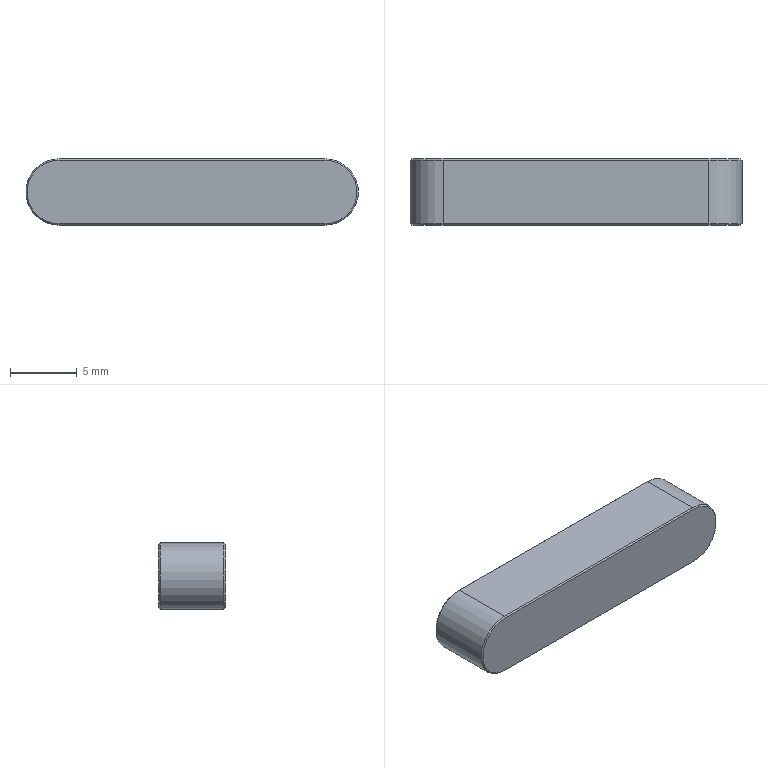Part | STEP file | Plain key type A 5x5x25 | 1 solid | 14 faces | box 25 x 5 x 5 mm | volume 597.62 mm3 | plane 8 | cone 4 | cylinder 2 | commonest cylinder face diameters 5 x2
STEP:
#1=CARTESIAN_POINT('',(0.,0.,0.));
#2=DIRECTION('',(0.,0.,1.));
#3=DIRECTION('',(1.,0.,0.));
#4=AXIS2_PLACEMENT_3D('',#1,#2,#3);
#5=CARTESIAN_POINT('',(-10.,2.4,-2.5));
#6=VERTEX_POINT('',#5);
#7=CARTESIAN_POINT('',(-10.,-2.4,-2.5));
#8=VERTEX_POINT('',#7);
#9=CARTESIAN_POINT('',(-10.,2.5,-2.5));
#10=DIRECTION('',(0.,-1.,0.));
#11=VECTOR('',#10,1.);
#12=LINE('',#9,#11);
#13=CARTESIAN_POINT('',(-10.,2.5,0.));
#14=DIRECTION('',(0.,-1.,0.));
#15=DIRECTION('',(0.,0.,-1.));
#16=AXIS2_PLACEMENT_3D('',#13,#14,#15);
#17=CYLINDRICAL_SURFACE('',#16,2.5);
#18=CARTESIAN_POINT('',(6.283,0.));
#19=DIRECTION('',(0.,1.));
#20=VECTOR('',#19,1.);
#21=LINE('',#18,#20);
#22=(GEOMETRIC_REPRESENTATION_CONTEXT(2)PARAMETRIC_REPRESENTATION_CONTEXT()REPRESENTATION_CONTEXT('',''));
#23=DEFINITIONAL_REPRESENTATION('',(#21),#22);
#24=PCURVE('',#17,#23);
#25=CARTESIAN_POINT('',(-10.,2.5,-2.5));
#26=DIRECTION('',(0.,0.,1.));
#27=DIRECTION('',(1.,0.,0.));
#28=AXIS2_PLACEMENT_3D('',#25,#26,#27);
#29=PLANE('',#28);
#30=CARTESIAN_POINT('',(0.,0.));
#31=DIRECTION('',(0.,-1.));
#32=VECTOR('',#31,1.);
#33=LINE('',#30,#32);
#34=(GEOMETRIC_REPRESENTATION_CONTEXT(2)PARAMETRIC_REPRESENTATION_CONTEXT()REPRESENTATION_CONTEXT('',''));
#35=DEFINITIONAL_REPRESENTATION('',(#33),#34);
#36=PCURVE('',#29,#35);
#37=SURFACE_CURVE('',#12,(#24,#36),.PCURVE_S1.);
#38=EDGE_CURVE('',#6,#8,#37,.T.);
#39=ORIENTED_EDGE('',*,*,#38,.T.);
#40=CARTESIAN_POINT('',(-10.,-2.4,2.5));
#41=VERTEX_POINT('',#40);
#42=CARTESIAN_POINT('',(-10.,-2.4,0.));
#43=DIRECTION('',(0.,1.,0.));
#44=DIRECTION('',(0.,0.,1.));
#45=AXIS2_PLACEMENT_3D('',#42,#43,#44);
#46=CIRCLE('',#45,2.5);
#47=CARTESIAN_POINT('',(9.425,4.9));
#48=DIRECTION('',(-1.,0.));
#49=VECTOR('',#48,1.);
#50=LINE('',#47,#49);
#51=(GEOMETRIC_REPRESENTATION_CONTEXT(2)PARAMETRIC_REPRESENTATION_CONTEXT()REPRESENTATION_CONTEXT('',''));
#52=DEFINITIONAL_REPRESENTATION('',(#50),#51);
#53=PCURVE('',#17,#52);
#54=CARTESIAN_POINT('',(-10.,-2.4,0.));
#55=DIRECTION('',(0.,1.,0.));
#56=DIRECTION('',(0.,0.,1.));
#57=AXIS2_PLACEMENT_3D('',#54,#55,#56);
#58=CONICAL_SURFACE('',#57,2.5,0.7854);
#59=CARTESIAN_POINT('',(0.,0.));
#60=DIRECTION('',(1.,0.));
#61=VECTOR('',#60,1.);
#62=LINE('',#59,#61);
#63=(GEOMETRIC_REPRESENTATION_CONTEXT(2)PARAMETRIC_REPRESENTATION_CONTEXT()REPRESENTATION_CONTEXT('',''));
#64=DEFINITIONAL_REPRESENTATION('',(#62),#63);
#65=PCURVE('',#58,#64);
#66=SURFACE_CURVE('',#46,(#53,#65),.PCURVE_S1.);
#67=EDGE_CURVE('',#8,#41,#66,.T.);
#68=ORIENTED_EDGE('',*,*,#67,.T.);
#69=CARTESIAN_POINT('',(-10.,2.4,2.5));
#70=VERTEX_POINT('',#69);
#71=CARTESIAN_POINT('',(-10.,2.5,2.5));
#72=DIRECTION('',(0.,-1.,0.));
#73=VECTOR('',#72,1.);
#74=LINE('',#71,#73);
#75=CARTESIAN_POINT('',(3.142,0.));
#76=DIRECTION('',(0.,1.));
#77=VECTOR('',#76,1.);
#78=LINE('',#75,#77);
#79=(GEOMETRIC_REPRESENTATION_CONTEXT(2)PARAMETRIC_REPRESENTATION_CONTEXT()REPRESENTATION_CONTEXT('',''));
#80=DEFINITIONAL_REPRESENTATION('',(#78),#79);
#81=PCURVE('',#17,#80);
#82=CARTESIAN_POINT('',(-10.,2.5,2.5));
#83=DIRECTION('',(0.,0.,-1.));
#84=DIRECTION('',(-1.,0.,0.));
#85=AXIS2_PLACEMENT_3D('',#82,#83,#84);
#86=PLANE('',#85);
#87=CARTESIAN_POINT('',(0.,0.));
#88=DIRECTION('',(0.,-1.));
#89=VECTOR('',#88,1.);
#90=LINE('',#87,#89);
#91=(GEOMETRIC_REPRESENTATION_CONTEXT(2)PARAMETRIC_REPRESENTATION_CONTEXT()REPRESENTATION_CONTEXT('',''));
#92=DEFINITIONAL_REPRESENTATION('',(#90),#91);
#93=PCURVE('',#86,#92);
#94=SURFACE_CURVE('',#74,(#81,#93),.PCURVE_S1.);
#95=EDGE_CURVE('',#70,#41,#94,.T.);
#96=ORIENTED_EDGE('',*,*,#95,.F.);
#97=CARTESIAN_POINT('',(-10.,2.4,0.));
#98=DIRECTION('',(0.,-1.,0.));
#99=DIRECTION('',(0.,0.,1.));
#100=AXIS2_PLACEMENT_3D('',#97,#98,#99);
#101=CIRCLE('',#100,2.5);
#102=CARTESIAN_POINT('',(3.142,0.1));
#103=DIRECTION('',(1.,0.));
#104=VECTOR('',#103,1.);
#105=LINE('',#102,#104);
#106=(GEOMETRIC_REPRESENTATION_CONTEXT(2)PARAMETRIC_REPRESENTATION_CONTEXT()REPRESENTATION_CONTEXT('',''));
#107=DEFINITIONAL_REPRESENTATION('',(#105),#106);
#108=PCURVE('',#17,#107);
#109=CARTESIAN_POINT('',(-10.,2.5,0.));
#110=DIRECTION('',(0.,-1.,0.));
#111=DIRECTION('',(0.,0.,-1.));
#112=AXIS2_PLACEMENT_3D('',#109,#110,#111);
#113=CONICAL_SURFACE('',#112,2.4,0.7854);
#114=CARTESIAN_POINT('',(3.142,0.1));
#115=DIRECTION('',(1.,0.));
#116=VECTOR('',#115,1.);
#117=LINE('',#114,#116);
#118=(GEOMETRIC_REPRESENTATION_CONTEXT(2)PARAMETRIC_REPRESENTATION_CONTEXT()REPRESENTATION_CONTEXT('',''));
#119=DEFINITIONAL_REPRESENTATION('',(#117),#118);
#120=PCURVE('',#113,#119);
#121=SURFACE_CURVE('',#101,(#108,#120),.PCURVE_S1.);
#122=EDGE_CURVE('',#70,#6,#121,.T.);
#123=ORIENTED_EDGE('',*,*,#122,.T.);
#124=EDGE_LOOP('',(#39,#68,#96,#123));
#125=FACE_BOUND('',#124,.T.);
#126=ADVANCED_FACE('',(#125),#17,.T.);
#127=ORIENTED_EDGE('',*,*,#95,.T.);
#128=CARTESIAN_POINT('',(10.,-2.4,2.5));
#129=VERTEX_POINT('',#128);
#130=CARTESIAN_POINT('',(-10.,-2.4,2.5));
#131=DIRECTION('',(1.,0.,0.));
#132=VECTOR('',#131,1.);
#133=LINE('',#130,#132);
#134=CARTESIAN_POINT('',(0.,-4.9));
#135=DIRECTION('',(-1.,0.));
#136=VECTOR('',#135,1.);
#137=LINE('',#134,#136);
#138=(GEOMETRIC_REPRESENTATION_CONTEXT(2)PARAMETRIC_REPRESENTATION_CONTEXT()REPRESENTATION_CONTEXT('',''));
#139=DEFINITIONAL_REPRESENTATION('',(#137),#138);
#140=PCURVE('',#86,#139);
#141=CARTESIAN_POINT('',(-10.,-2.4,2.5));
#142=DIRECTION('',(0.,0.7071,-0.7071));
#143=DIRECTION('',(1.,0.,0.));
#144=AXIS2_PLACEMENT_3D('',#141,#142,#143);
#145=PLANE('',#144);
#146=CARTESIAN_POINT('',(0.,0.));
#147=DIRECTION('',(1.,0.));
#148=VECTOR('',#147,1.);
#149=LINE('',#146,#148);
#150=(GEOMETRIC_REPRESENTATION_CONTEXT(2)PARAMETRIC_REPRESENTATION_CONTEXT()REPRESENTATION_CONTEXT('',''));
#151=DEFINITIONAL_REPRESENTATION('',(#149),#150);
#152=PCURVE('',#145,#151);
#153=SURFACE_CURVE('',#133,(#140,#152),.PCURVE_S1.);
#154=EDGE_CURVE('',#41,#129,#153,.T.);
#155=ORIENTED_EDGE('',*,*,#154,.T.);
#156=CARTESIAN_POINT('',(10.,2.4,2.5));
#157=VERTEX_POINT('',#156);
#158=CARTESIAN_POINT('',(10.,2.5,2.5));
#159=DIRECTION('',(0.,-1.,0.));
#160=VECTOR('',#159,1.);
#161=LINE('',#158,#160);
#162=CARTESIAN_POINT('',(-20.,0.));
#163=DIRECTION('',(0.,-1.));
#164=VECTOR('',#163,1.);
#165=LINE('',#162,#164);
#166=(GEOMETRIC_REPRESENTATION_CONTEXT(2)PARAMETRIC_REPRESENTATION_CONTEXT()REPRESENTATION_CONTEXT('',''));
#167=DEFINITIONAL_REPRESENTATION('',(#165),#166);
#168=PCURVE('',#86,#167);
#169=CARTESIAN_POINT('',(10.,2.5,0.));
#170=DIRECTION('',(0.,-1.,0.));
#171=DIRECTION('',(0.,0.,-1.));
#172=AXIS2_PLACEMENT_3D('',#169,#170,#171);
#173=CYLINDRICAL_SURFACE('',#172,2.5);
#174=CARTESIAN_POINT('',(3.142,0.));
#175=DIRECTION('',(0.,1.));
#176=VECTOR('',#175,1.);
#177=LINE('',#174,#176);
#178=(GEOMETRIC_REPRESENTATION_CONTEXT(2)PARAMETRIC_REPRESENTATION_CONTEXT()REPRESENTATION_CONTEXT('',''));
#179=DEFINITIONAL_REPRESENTATION('',(#177),#178);
#180=PCURVE('',#173,#179);
#181=SURFACE_CURVE('',#161,(#168,#180),.PCURVE_S1.);
#182=EDGE_CURVE('',#157,#129,#181,.T.);
#183=ORIENTED_EDGE('',*,*,#182,.F.);
#184=CARTESIAN_POINT('',(-10.,2.4,2.5));
#185=DIRECTION('',(-1.,0.,0.));
#186=VECTOR('',#185,1.);
#187=LINE('',#184,#186);
#188=CARTESIAN_POINT('',(0.,-0.1));
#189=DIRECTION('',(1.,0.));
#190=VECTOR('',#189,1.);
#191=LINE('',#188,#190);
#192=(GEOMETRIC_REPRESENTATION_CONTEXT(2)PARAMETRIC_REPRESENTATION_CONTEXT()REPRESENTATION_CONTEXT('',''));
#193=DEFINITIONAL_REPRESENTATION('',(#191),#192);
#194=PCURVE('',#86,#193);
#195=CARTESIAN_POINT('',(-10.,2.5,2.4));
#196=DIRECTION('',(0.,0.7071,0.7071));
#197=DIRECTION('',(-1.,0.,0.));
#198=AXIS2_PLACEMENT_3D('',#195,#196,#197);
#199=PLANE('',#198);
#200=CARTESIAN_POINT('',(0.,0.1414));
#201=DIRECTION('',(1.,0.));
#202=VECTOR('',#201,1.);
#203=LINE('',#200,#202);
#204=(GEOMETRIC_REPRESENTATION_CONTEXT(2)PARAMETRIC_REPRESENTATION_CONTEXT()REPRESENTATION_CONTEXT('',''));
#205=DEFINITIONAL_REPRESENTATION('',(#203),#204);
#206=PCURVE('',#199,#205);
#207=SURFACE_CURVE('',#187,(#194,#206),.PCURVE_S1.);
#208=EDGE_CURVE('',#157,#70,#207,.T.);
#209=ORIENTED_EDGE('',*,*,#208,.T.);
#210=EDGE_LOOP('',(#127,#155,#183,#209));
#211=FACE_BOUND('',#210,.T.);
#212=ADVANCED_FACE('',(#211),#86,.F.);
#213=ORIENTED_EDGE('',*,*,#182,.T.);
#214=CARTESIAN_POINT('',(10.,-2.4,-2.5));
#215=VERTEX_POINT('',#214);
#216=CARTESIAN_POINT('',(10.,-2.4,0.));
#217=DIRECTION('',(0.,1.,0.));
#218=DIRECTION('',(0.,0.,1.));
#219=AXIS2_PLACEMENT_3D('',#216,#217,#218);
#220=CIRCLE('',#219,2.5);
#221=CARTESIAN_POINT('',(3.142,4.9));
#222=DIRECTION('',(-1.,0.));
#223=VECTOR('',#222,1.);
#224=LINE('',#221,#223);
#225=(GEOMETRIC_REPRESENTATION_CONTEXT(2)PARAMETRIC_REPRESENTATION_CONTEXT()REPRESENTATION_CONTEXT('',''));
#226=DEFINITIONAL_REPRESENTATION('',(#224),#225);
#227=PCURVE('',#173,#226);
#228=CARTESIAN_POINT('',(10.,-2.4,0.));
#229=DIRECTION('',(0.,1.,0.));
#230=DIRECTION('',(0.,0.,1.));
#231=AXIS2_PLACEMENT_3D('',#228,#229,#230);
#232=CONICAL_SURFACE('',#231,2.5,0.7854);
#233=CARTESIAN_POINT('',(0.,0.));
#234=DIRECTION('',(1.,0.));
#235=VECTOR('',#234,1.);
#236=LINE('',#233,#235);
#237=(GEOMETRIC_REPRESENTATION_CONTEXT(2)PARAMETRIC_REPRESENTATION_CONTEXT()REPRESENTATION_CONTEXT('',''));
#238=DEFINITIONAL_REPRESENTATION('',(#236),#237);
#239=PCURVE('',#232,#238);
#240=SURFACE_CURVE('',#220,(#227,#239),.PCURVE_S1.);
#241=EDGE_CURVE('',#129,#215,#240,.T.);
#242=ORIENTED_EDGE('',*,*,#241,.T.);
#243=CARTESIAN_POINT('',(10.,2.4,-2.5));
#244=VERTEX_POINT('',#243);
#245=CARTESIAN_POINT('',(10.,2.5,-2.5));
#246=DIRECTION('',(0.,-1.,0.));
#247=VECTOR('',#246,1.);
#248=LINE('',#245,#247);
#249=CARTESIAN_POINT('',(0.,0.));
#250=DIRECTION('',(0.,1.));
#251=VECTOR('',#250,1.);
#252=LINE('',#249,#251);
#253=(GEOMETRIC_REPRESENTATION_CONTEXT(2)PARAMETRIC_REPRESENTATION_CONTEXT()REPRESENTATION_CONTEXT('',''));
#254=DEFINITIONAL_REPRESENTATION('',(#252),#253);
#255=PCURVE('',#173,#254);
#256=CARTESIAN_POINT('',(20.,0.));
#257=DIRECTION('',(0.,-1.));
#258=VECTOR('',#257,1.);
#259=LINE('',#256,#258);
#260=(GEOMETRIC_REPRESENTATION_CONTEXT(2)PARAMETRIC_REPRESENTATION_CONTEXT()REPRESENTATION_CONTEXT('',''));
#261=DEFINITIONAL_REPRESENTATION('',(#259),#260);
#262=PCURVE('',#29,#261);
#263=SURFACE_CURVE('',#248,(#255,#262),.PCURVE_S1.);
#264=EDGE_CURVE('',#244,#215,#263,.T.);
#265=ORIENTED_EDGE('',*,*,#264,.F.);
#266=CARTESIAN_POINT('',(10.,2.4,0.));
#267=DIRECTION('',(0.,-1.,0.));
#268=DIRECTION('',(0.,0.,1.));
#269=AXIS2_PLACEMENT_3D('',#266,#267,#268);
#270=CIRCLE('',#269,2.5);
#271=CARTESIAN_POINT('',(-3.142,0.1));
#272=DIRECTION('',(1.,0.));
#273=VECTOR('',#272,1.);
#274=LINE('',#271,#273);
#275=(GEOMETRIC_REPRESENTATION_CONTEXT(2)PARAMETRIC_REPRESENTATION_CONTEXT()REPRESENTATION_CONTEXT('',''));
#276=DEFINITIONAL_REPRESENTATION('',(#274),#275);
#277=PCURVE('',#173,#276);
#278=CARTESIAN_POINT('',(10.,2.5,0.));
#279=DIRECTION('',(0.,-1.,0.));
#280=DIRECTION('',(0.,0.,-1.));
#281=AXIS2_PLACEMENT_3D('',#278,#279,#280);
#282=CONICAL_SURFACE('',#281,2.4,0.7854);
#283=CARTESIAN_POINT('',(-3.142,0.1));
#284=DIRECTION('',(1.,0.));
#285=VECTOR('',#284,1.);
#286=LINE('',#283,#285);
#287=(GEOMETRIC_REPRESENTATION_CONTEXT(2)PARAMETRIC_REPRESENTATION_CONTEXT()REPRESENTATION_CONTEXT('',''));
#288=DEFINITIONAL_REPRESENTATION('',(#286),#287);
#289=PCURVE('',#282,#288);
#290=SURFACE_CURVE('',#270,(#277,#289),.PCURVE_S1.);
#291=EDGE_CURVE('',#244,#157,#290,.T.);
#292=ORIENTED_EDGE('',*,*,#291,.T.);
#293=EDGE_LOOP('',(#213,#242,#265,#292));
#294=FACE_BOUND('',#293,.T.);
#295=ADVANCED_FACE('',(#294),#173,.T.);
#296=ORIENTED_EDGE('',*,*,#264,.T.);
#297=CARTESIAN_POINT('',(-10.,-2.4,-2.5));
#298=DIRECTION('',(-1.,0.,0.));
#299=VECTOR('',#298,1.);
#300=LINE('',#297,#299);
#301=CARTESIAN_POINT('',(0.,-4.9));
#302=DIRECTION('',(-1.,0.));
#303=VECTOR('',#302,1.);
#304=LINE('',#301,#303);
#305=(GEOMETRIC_REPRESENTATION_CONTEXT(2)PARAMETRIC_REPRESENTATION_CONTEXT()REPRESENTATION_CONTEXT('',''));
#306=DEFINITIONAL_REPRESENTATION('',(#304),#305);
#307=PCURVE('',#29,#306);
#308=CARTESIAN_POINT('',(-10.,-2.4,-2.5));
#309=DIRECTION('',(0.,0.7071,0.7071));
#310=DIRECTION('',(-1.,0.,0.));
#311=AXIS2_PLACEMENT_3D('',#308,#309,#310);
#312=PLANE('',#311);
#313=CARTESIAN_POINT('',(0.,0.));
#314=DIRECTION('',(1.,0.));
#315=VECTOR('',#314,1.);
#316=LINE('',#313,#315);
#317=(GEOMETRIC_REPRESENTATION_CONTEXT(2)PARAMETRIC_REPRESENTATION_CONTEXT()REPRESENTATION_CONTEXT('',''));
#318=DEFINITIONAL_REPRESENTATION('',(#316),#317);
#319=PCURVE('',#312,#318);
#320=SURFACE_CURVE('',#300,(#307,#319),.PCURVE_S1.);
#321=EDGE_CURVE('',#215,#8,#320,.T.);
#322=ORIENTED_EDGE('',*,*,#321,.T.);
#323=ORIENTED_EDGE('',*,*,#38,.F.);
#324=CARTESIAN_POINT('',(10.,2.4,-2.5));
#325=DIRECTION('',(1.,0.,0.));
#326=VECTOR('',#325,1.);
#327=LINE('',#324,#326);
#328=CARTESIAN_POINT('',(20.,-0.1));
#329=DIRECTION('',(1.,0.));
#330=VECTOR('',#329,1.);
#331=LINE('',#328,#330);
#332=(GEOMETRIC_REPRESENTATION_CONTEXT(2)PARAMETRIC_REPRESENTATION_CONTEXT()REPRESENTATION_CONTEXT('',''));
#333=DEFINITIONAL_REPRESENTATION('',(#331),#332);
#334=PCURVE('',#29,#333);
#335=CARTESIAN_POINT('',(-10.,2.5,-2.4));
#336=DIRECTION('',(0.,0.7071,-0.7071));
#337=DIRECTION('',(1.,0.,0.));
#338=AXIS2_PLACEMENT_3D('',#335,#336,#337);
#339=PLANE('',#338);
#340=CARTESIAN_POINT('',(20.,0.1414));
#341=DIRECTION('',(1.,0.));
#342=VECTOR('',#341,1.);
#343=LINE('',#340,#342);
#344=(GEOMETRIC_REPRESENTATION_CONTEXT(2)PARAMETRIC_REPRESENTATION_CONTEXT()REPRESENTATION_CONTEXT('',''));
#345=DEFINITIONAL_REPRESENTATION('',(#343),#344);
#346=PCURVE('',#339,#345);
#347=SURFACE_CURVE('',#327,(#334,#346),.PCURVE_S1.);
#348=EDGE_CURVE('',#6,#244,#347,.T.);
#349=ORIENTED_EDGE('',*,*,#348,.T.);
#350=EDGE_LOOP('',(#296,#322,#323,#349));
#351=FACE_BOUND('',#350,.T.);
#352=ADVANCED_FACE('',(#351),#29,.F.);
#353=CARTESIAN_POINT('',(-10.,2.5,-2.4));
#354=VERTEX_POINT('',#353);
#355=CARTESIAN_POINT('',(-10.,2.5,2.4));
#356=VERTEX_POINT('',#355);
#357=CARTESIAN_POINT('',(-10.,2.5,0.));
#358=DIRECTION('',(0.,1.,0.));
#359=DIRECTION('',(0.,0.,1.));
#360=AXIS2_PLACEMENT_3D('',#357,#358,#359);
#361=CIRCLE('',#360,2.4);
#362=CARTESIAN_POINT('',(-10.,2.5,0.));
#363=DIRECTION('',(0.,1.,0.));
#364=DIRECTION('',(0.,0.,1.));
#365=AXIS2_PLACEMENT_3D('',#362,#363,#364);
#366=PLANE('',#365);
#367=CARTESIAN_POINT('',(0.,0.));
#368=DIRECTION('',(1.,0.));
#369=AXIS2_PLACEMENT_2D('',#367,#368);
#370=CIRCLE('',#369,2.4);
#371=(GEOMETRIC_REPRESENTATION_CONTEXT(2)PARAMETRIC_REPRESENTATION_CONTEXT()REPRESENTATION_CONTEXT('',''));
#372=DEFINITIONAL_REPRESENTATION('',(#370),#371);
#373=PCURVE('',#366,#372);
#374=CARTESIAN_POINT('',(9.425,0.));
#375=DIRECTION('',(-1.,0.));
#376=VECTOR('',#375,1.);
#377=LINE('',#374,#376);
#378=(GEOMETRIC_REPRESENTATION_CONTEXT(2)PARAMETRIC_REPRESENTATION_CONTEXT()REPRESENTATION_CONTEXT('',''));
#379=DEFINITIONAL_REPRESENTATION('',(#377),#378);
#380=PCURVE('',#113,#379);
#381=SURFACE_CURVE('',#361,(#373,#380),.PCURVE_S1.);
#382=EDGE_CURVE('',#354,#356,#381,.T.);
#383=ORIENTED_EDGE('',*,*,#382,.T.);
#384=CARTESIAN_POINT('',(10.,2.5,2.4));
#385=VERTEX_POINT('',#384);
#386=CARTESIAN_POINT('',(10.,2.5,2.4));
#387=DIRECTION('',(1.,0.,0.));
#388=VECTOR('',#387,1.);
#389=LINE('',#386,#388);
#390=CARTESIAN_POINT('',(2.4,20.));
#391=DIRECTION('',(0.,1.));
#392=VECTOR('',#391,1.);
#393=LINE('',#390,#392);
#394=(GEOMETRIC_REPRESENTATION_CONTEXT(2)PARAMETRIC_REPRESENTATION_CONTEXT()REPRESENTATION_CONTEXT('',''));
#395=DEFINITIONAL_REPRESENTATION('',(#393),#394);
#396=PCURVE('',#366,#395);
#397=CARTESIAN_POINT('',(-20.,0.));
#398=DIRECTION('',(-1.,0.));
#399=VECTOR('',#398,1.);
#400=LINE('',#397,#399);
#401=(GEOMETRIC_REPRESENTATION_CONTEXT(2)PARAMETRIC_REPRESENTATION_CONTEXT()REPRESENTATION_CONTEXT('',''));
#402=DEFINITIONAL_REPRESENTATION('',(#400),#401);
#403=PCURVE('',#199,#402);
#404=SURFACE_CURVE('',#389,(#396,#403),.PCURVE_S1.);
#405=EDGE_CURVE('',#356,#385,#404,.T.);
#406=ORIENTED_EDGE('',*,*,#405,.T.);
#407=CARTESIAN_POINT('',(10.,2.5,-2.4));
#408=VERTEX_POINT('',#407);
#409=CARTESIAN_POINT('',(10.,2.5,0.));
#410=DIRECTION('',(0.,1.,0.));
#411=DIRECTION('',(0.,0.,1.));
#412=AXIS2_PLACEMENT_3D('',#409,#410,#411);
#413=CIRCLE('',#412,2.4);
#414=CARTESIAN_POINT('',(0.,20.));
#415=DIRECTION('',(1.,0.));
#416=AXIS2_PLACEMENT_2D('',#414,#415);
#417=CIRCLE('',#416,2.4);
#418=(GEOMETRIC_REPRESENTATION_CONTEXT(2)PARAMETRIC_REPRESENTATION_CONTEXT()REPRESENTATION_CONTEXT('',''));
#419=DEFINITIONAL_REPRESENTATION('',(#417),#418);
#420=PCURVE('',#366,#419);
#421=CARTESIAN_POINT('',(3.142,0.));
#422=DIRECTION('',(-1.,0.));
#423=VECTOR('',#422,1.);
#424=LINE('',#421,#423);
#425=(GEOMETRIC_REPRESENTATION_CONTEXT(2)PARAMETRIC_REPRESENTATION_CONTEXT()REPRESENTATION_CONTEXT('',''));
#426=DEFINITIONAL_REPRESENTATION('',(#424),#425);
#427=PCURVE('',#282,#426);
#428=SURFACE_CURVE('',#413,(#420,#427),.PCURVE_S1.);
#429=EDGE_CURVE('',#385,#408,#428,.T.);
#430=ORIENTED_EDGE('',*,*,#429,.T.);
#431=CARTESIAN_POINT('',(-10.,2.5,-2.4));
#432=DIRECTION('',(-1.,0.,0.));
#433=VECTOR('',#432,1.);
#434=LINE('',#431,#433);
#435=CARTESIAN_POINT('',(-2.4,0.));
#436=DIRECTION('',(0.,-1.));
#437=VECTOR('',#436,1.);
#438=LINE('',#435,#437);
#439=(GEOMETRIC_REPRESENTATION_CONTEXT(2)PARAMETRIC_REPRESENTATION_CONTEXT()REPRESENTATION_CONTEXT('',''));
#440=DEFINITIONAL_REPRESENTATION('',(#438),#439);
#441=PCURVE('',#366,#440);
#442=CARTESIAN_POINT('',(0.,0.));
#443=DIRECTION('',(-1.,0.));
#444=VECTOR('',#443,1.);
#445=LINE('',#442,#444);
#446=(GEOMETRIC_REPRESENTATION_CONTEXT(2)PARAMETRIC_REPRESENTATION_CONTEXT()REPRESENTATION_CONTEXT('',''));
#447=DEFINITIONAL_REPRESENTATION('',(#445),#446);
#448=PCURVE('',#339,#447);
#449=SURFACE_CURVE('',#434,(#441,#448),.PCURVE_S1.);
#450=EDGE_CURVE('',#408,#354,#449,.T.);
#451=ORIENTED_EDGE('',*,*,#450,.T.);
#452=EDGE_LOOP('',(#383,#406,#430,#451));
#453=FACE_BOUND('',#452,.T.);
#454=ADVANCED_FACE('',(#453),#366,.T.);
#455=CARTESIAN_POINT('',(10.,-2.5,-2.4));
#456=VERTEX_POINT('',#455);
#457=CARTESIAN_POINT('',(10.,-2.5,2.4));
#458=VERTEX_POINT('',#457);
#459=CARTESIAN_POINT('',(10.,-2.5,0.));
#460=DIRECTION('',(0.,-1.,0.));
#461=DIRECTION('',(0.,0.,1.));
#462=AXIS2_PLACEMENT_3D('',#459,#460,#461);
#463=CIRCLE('',#462,2.4);
#464=CARTESIAN_POINT('',(-10.,-2.5,0.));
#465=DIRECTION('',(0.,1.,0.));
#466=DIRECTION('',(0.,0.,1.));
#467=AXIS2_PLACEMENT_3D('',#464,#465,#466);
#468=PLANE('',#467);
#469=CARTESIAN_POINT('',(2.4,20.));
#470=CARTESIAN_POINT('',(2.4,15.843));
#471=CARTESIAN_POINT('',(-1.2,17.922));
#472=CARTESIAN_POINT('',(-4.8,20.));
#473=CARTESIAN_POINT('',(-1.2,22.078));
#474=CARTESIAN_POINT('',(2.4,24.157));
#475=CARTESIAN_POINT('',(2.4,20.));
#476=(BOUNDED_CURVE()B_SPLINE_CURVE(2,(#469,#470,#471,#472,#473,#474,#475),.UNSPECIFIED.,.T.,.F.)B_SPLINE_CURVE_WITH_KNOTS((1,2,2,2,2,1),(-2.094,0.,2.094,4.189,6.283,8.378),.UNSPECIFIED.)CURVE()GEOMETRIC_REPRESENTATION_ITEM()RATIONAL_B_SPLINE_CURVE((1.,0.5,1.,0.5,1.,0.5,1.))REPRESENTATION_ITEM(''));
#477=(GEOMETRIC_REPRESENTATION_CONTEXT(2)PARAMETRIC_REPRESENTATION_CONTEXT()REPRESENTATION_CONTEXT('',''));
#478=DEFINITIONAL_REPRESENTATION('',(#476),#477);
#479=PCURVE('',#468,#478);
#480=CARTESIAN_POINT('',(6.283,-0.1));
#481=DIRECTION('',(-1.,0.));
#482=VECTOR('',#481,1.);
#483=LINE('',#480,#482);
#484=(GEOMETRIC_REPRESENTATION_CONTEXT(2)PARAMETRIC_REPRESENTATION_CONTEXT()REPRESENTATION_CONTEXT('',''));
#485=DEFINITIONAL_REPRESENTATION('',(#483),#484);
#486=PCURVE('',#232,#485);
#487=SURFACE_CURVE('',#463,(#479,#486),.PCURVE_S1.);
#488=EDGE_CURVE('',#456,#458,#487,.T.);
#489=ORIENTED_EDGE('',*,*,#488,.T.);
#490=CARTESIAN_POINT('',(-10.,-2.5,2.4));
#491=VERTEX_POINT('',#490);
#492=CARTESIAN_POINT('',(-10.,-2.5,2.4));
#493=DIRECTION('',(-1.,0.,0.));
#494=VECTOR('',#493,1.);
#495=LINE('',#492,#494);
#496=CARTESIAN_POINT('',(2.4,0.));
#497=DIRECTION('',(0.,-1.));
#498=VECTOR('',#497,1.);
#499=LINE('',#496,#498);
#500=(GEOMETRIC_REPRESENTATION_CONTEXT(2)PARAMETRIC_REPRESENTATION_CONTEXT()REPRESENTATION_CONTEXT('',''));
#501=DEFINITIONAL_REPRESENTATION('',(#499),#500);
#502=PCURVE('',#468,#501);
#503=CARTESIAN_POINT('',(0.,0.1414));
#504=DIRECTION('',(-1.,0.));
#505=VECTOR('',#504,1.);
#506=LINE('',#503,#505);
#507=(GEOMETRIC_REPRESENTATION_CONTEXT(2)PARAMETRIC_REPRESENTATION_CONTEXT()REPRESENTATION_CONTEXT('',''));
#508=DEFINITIONAL_REPRESENTATION('',(#506),#507);
#509=PCURVE('',#145,#508);
#510=SURFACE_CURVE('',#495,(#502,#509),.PCURVE_S1.);
#511=EDGE_CURVE('',#458,#491,#510,.T.);
#512=ORIENTED_EDGE('',*,*,#511,.T.);
#513=CARTESIAN_POINT('',(-10.,-2.5,-2.4));
#514=VERTEX_POINT('',#513);
#515=CARTESIAN_POINT('',(-10.,-2.5,0.));
#516=DIRECTION('',(0.,-1.,0.));
#517=DIRECTION('',(0.,0.,1.));
#518=AXIS2_PLACEMENT_3D('',#515,#516,#517);
#519=CIRCLE('',#518,2.4);
#520=CARTESIAN_POINT('',(2.4,0.));
#521=CARTESIAN_POINT('',(2.4,-4.157));
#522=CARTESIAN_POINT('',(-1.2,-2.078));
#523=CARTESIAN_POINT('',(-4.8,0.));
#524=CARTESIAN_POINT('',(-1.2,2.078));
#525=CARTESIAN_POINT('',(2.4,4.157));
#526=CARTESIAN_POINT('',(2.4,0.));
#527=(BOUNDED_CURVE()B_SPLINE_CURVE(2,(#520,#521,#522,#523,#524,#525,#526),.UNSPECIFIED.,.T.,.F.)B_SPLINE_CURVE_WITH_KNOTS((1,2,2,2,2,1),(-2.094,0.,2.094,4.189,6.283,8.378),.UNSPECIFIED.)CURVE()GEOMETRIC_REPRESENTATION_ITEM()RATIONAL_B_SPLINE_CURVE((1.,0.5,1.,0.5,1.,0.5,1.))REPRESENTATION_ITEM(''));
#528=(GEOMETRIC_REPRESENTATION_CONTEXT(2)PARAMETRIC_REPRESENTATION_CONTEXT()REPRESENTATION_CONTEXT('',''));
#529=DEFINITIONAL_REPRESENTATION('',(#527),#528);
#530=PCURVE('',#468,#529);
#531=CARTESIAN_POINT('',(6.283,-0.1));
#532=DIRECTION('',(-1.,0.));
#533=VECTOR('',#532,1.);
#534=LINE('',#531,#533);
#535=(GEOMETRIC_REPRESENTATION_CONTEXT(2)PARAMETRIC_REPRESENTATION_CONTEXT()REPRESENTATION_CONTEXT('',''));
#536=DEFINITIONAL_REPRESENTATION('',(#534),#535);
#537=PCURVE('',#58,#536);
#538=SURFACE_CURVE('',#519,(#530,#537),.PCURVE_S1.);
#539=EDGE_CURVE('',#491,#514,#538,.T.);
#540=ORIENTED_EDGE('',*,*,#539,.T.);
#541=CARTESIAN_POINT('',(-10.,-2.5,-2.4));
#542=DIRECTION('',(1.,0.,0.));
#543=VECTOR('',#542,1.);
#544=LINE('',#541,#543);
#545=CARTESIAN_POINT('',(-2.4,0.));
#546=DIRECTION('',(0.,1.));
#547=VECTOR('',#546,1.);
#548=LINE('',#545,#547);
#549=(GEOMETRIC_REPRESENTATION_CONTEXT(2)PARAMETRIC_REPRESENTATION_CONTEXT()REPRESENTATION_CONTEXT('',''));
#550=DEFINITIONAL_REPRESENTATION('',(#548),#549);
#551=PCURVE('',#468,#550);
#552=CARTESIAN_POINT('',(0.,0.1414));
#553=DIRECTION('',(-1.,0.));
#554=VECTOR('',#553,1.);
#555=LINE('',#552,#554);
#556=(GEOMETRIC_REPRESENTATION_CONTEXT(2)PARAMETRIC_REPRESENTATION_CONTEXT()REPRESENTATION_CONTEXT('',''));
#557=DEFINITIONAL_REPRESENTATION('',(#555),#556);
#558=PCURVE('',#312,#557);
#559=SURFACE_CURVE('',#544,(#551,#558),.PCURVE_S1.);
#560=EDGE_CURVE('',#514,#456,#559,.T.);
#561=ORIENTED_EDGE('',*,*,#560,.T.);
#562=EDGE_LOOP('',(#489,#512,#540,#561));
#563=FACE_BOUND('',#562,.T.);
#564=ADVANCED_FACE('',(#563),#468,.F.);
#565=CARTESIAN_POINT('',(10.,-2.5,-2.4));
#566=DIRECTION('',(0.,0.7071,-0.7071));
#567=VECTOR('',#566,1.);
#568=LINE('',#565,#567);
#569=CARTESIAN_POINT('',(-20.,0.1414));
#570=DIRECTION('',(0.,-1.));
#571=VECTOR('',#570,1.);
#572=LINE('',#569,#571);
#573=(GEOMETRIC_REPRESENTATION_CONTEXT(2)PARAMETRIC_REPRESENTATION_CONTEXT()REPRESENTATION_CONTEXT('',''));
#574=DEFINITIONAL_REPRESENTATION('',(#572),#573);
#575=PCURVE('',#312,#574);
#576=CARTESIAN_POINT('',(3.142,-0.1));
#577=DIRECTION('',(0.,1.));
#578=VECTOR('',#577,1.);
#579=LINE('',#576,#578);
#580=(GEOMETRIC_REPRESENTATION_CONTEXT(2)PARAMETRIC_REPRESENTATION_CONTEXT()REPRESENTATION_CONTEXT('',''));
#581=DEFINITIONAL_REPRESENTATION('',(#579),#580);
#582=PCURVE('',#232,#581);
#583=SURFACE_CURVE('',#568,(#575,#582),.PCURVE_S1.);
#584=EDGE_CURVE('',#456,#215,#583,.T.);
#585=ORIENTED_EDGE('',*,*,#584,.F.);
#586=ORIENTED_EDGE('',*,*,#560,.F.);
#587=CARTESIAN_POINT('',(-10.,-2.4,-2.5));
#588=DIRECTION('',(0.,-0.7071,0.7071));
#589=VECTOR('',#588,1.);
#590=LINE('',#587,#589);
#591=CARTESIAN_POINT('',(0.,0.));
#592=DIRECTION('',(0.,1.));
#593=VECTOR('',#592,1.);
#594=LINE('',#591,#593);
#595=(GEOMETRIC_REPRESENTATION_CONTEXT(2)PARAMETRIC_REPRESENTATION_CONTEXT()REPRESENTATION_CONTEXT('',''));
#596=DEFINITIONAL_REPRESENTATION('',(#594),#595);
#597=PCURVE('',#312,#596);
#598=CARTESIAN_POINT('',(3.142,0.));
#599=DIRECTION('',(0.,-1.));
#600=VECTOR('',#599,1.);
#601=LINE('',#598,#600);
#602=(GEOMETRIC_REPRESENTATION_CONTEXT(2)PARAMETRIC_REPRESENTATION_CONTEXT()REPRESENTATION_CONTEXT('',''));
#603=DEFINITIONAL_REPRESENTATION('',(#601),#602);
#604=PCURVE('',#58,#603);
#605=SURFACE_CURVE('',#590,(#597,#604),.PCURVE_S1.);
#606=EDGE_CURVE('',#8,#514,#605,.T.);
#607=ORIENTED_EDGE('',*,*,#606,.F.);
#608=ORIENTED_EDGE('',*,*,#321,.F.);
#609=EDGE_LOOP('',(#585,#586,#607,#608));
#610=FACE_BOUND('',#609,.T.);
#611=ADVANCED_FACE('',(#610),#312,.F.);
#612=ORIENTED_EDGE('',*,*,#606,.T.);
#613=ORIENTED_EDGE('',*,*,#539,.F.);
#614=CARTESIAN_POINT('',(-10.,-2.4,2.5));
#615=DIRECTION('',(0.,-0.7071,-0.7071));
#616=VECTOR('',#615,1.);
#617=LINE('',#614,#616);
#618=CARTESIAN_POINT('',(6.283,0.));
#619=DIRECTION('',(0.,-1.));
#620=VECTOR('',#619,1.);
#621=LINE('',#618,#620);
#622=(GEOMETRIC_REPRESENTATION_CONTEXT(2)PARAMETRIC_REPRESENTATION_CONTEXT()REPRESENTATION_CONTEXT('',''));
#623=DEFINITIONAL_REPRESENTATION('',(#621),#622);
#624=PCURVE('',#58,#623);
#625=CARTESIAN_POINT('',(0.,0.));
#626=DIRECTION('',(0.,1.));
#627=VECTOR('',#626,1.);
#628=LINE('',#625,#627);
#629=(GEOMETRIC_REPRESENTATION_CONTEXT(2)PARAMETRIC_REPRESENTATION_CONTEXT()REPRESENTATION_CONTEXT('',''));
#630=DEFINITIONAL_REPRESENTATION('',(#628),#629);
#631=PCURVE('',#145,#630);
#632=SURFACE_CURVE('',#617,(#624,#631),.PCURVE_S1.);
#633=EDGE_CURVE('',#41,#491,#632,.T.);
#634=ORIENTED_EDGE('',*,*,#633,.F.);
#635=ORIENTED_EDGE('',*,*,#67,.F.);
#636=EDGE_LOOP('',(#612,#613,#634,#635));
#637=FACE_BOUND('',#636,.T.);
#638=ADVANCED_FACE('',(#637),#58,.T.);
#639=ORIENTED_EDGE('',*,*,#584,.T.);
#640=ORIENTED_EDGE('',*,*,#241,.F.);
#641=CARTESIAN_POINT('',(10.,-2.5,2.4));
#642=DIRECTION('',(0.,0.7071,0.7071));
#643=VECTOR('',#642,1.);
#644=LINE('',#641,#643);
#645=CARTESIAN_POINT('',(0.,-0.1));
#646=DIRECTION('',(0.,1.));
#647=VECTOR('',#646,1.);
#648=LINE('',#645,#647);
#649=(GEOMETRIC_REPRESENTATION_CONTEXT(2)PARAMETRIC_REPRESENTATION_CONTEXT()REPRESENTATION_CONTEXT('',''));
#650=DEFINITIONAL_REPRESENTATION('',(#648),#649);
#651=PCURVE('',#232,#650);
#652=CARTESIAN_POINT('',(20.,0.1414));
#653=DIRECTION('',(0.,-1.));
#654=VECTOR('',#653,1.);
#655=LINE('',#652,#654);
#656=(GEOMETRIC_REPRESENTATION_CONTEXT(2)PARAMETRIC_REPRESENTATION_CONTEXT()REPRESENTATION_CONTEXT('',''));
#657=DEFINITIONAL_REPRESENTATION('',(#655),#656);
#658=PCURVE('',#145,#657);
#659=SURFACE_CURVE('',#644,(#651,#658),.PCURVE_S1.);
#660=EDGE_CURVE('',#458,#129,#659,.T.);
#661=ORIENTED_EDGE('',*,*,#660,.F.);
#662=ORIENTED_EDGE('',*,*,#488,.F.);
#663=EDGE_LOOP('',(#639,#640,#661,#662));
#664=FACE_BOUND('',#663,.T.);
#665=ADVANCED_FACE('',(#664),#232,.T.);
#666=ORIENTED_EDGE('',*,*,#633,.T.);
#667=ORIENTED_EDGE('',*,*,#511,.F.);
#668=ORIENTED_EDGE('',*,*,#660,.T.);
#669=ORIENTED_EDGE('',*,*,#154,.F.);
#670=EDGE_LOOP('',(#666,#667,#668,#669));
#671=FACE_BOUND('',#670,.T.);
#672=ADVANCED_FACE('',(#671),#145,.F.);
#673=CARTESIAN_POINT('',(10.,2.4,-2.5));
#674=DIRECTION('',(0.,0.7071,0.7071));
#675=VECTOR('',#674,1.);
#676=LINE('',#673,#675);
#677=CARTESIAN_POINT('',(20.,0.1414));
#678=DIRECTION('',(0.,-1.));
#679=VECTOR('',#678,1.);
#680=LINE('',#677,#679);
#681=(GEOMETRIC_REPRESENTATION_CONTEXT(2)PARAMETRIC_REPRESENTATION_CONTEXT()REPRESENTATION_CONTEXT('',''));
#682=DEFINITIONAL_REPRESENTATION('',(#680),#681);
#683=PCURVE('',#339,#682);
#684=CARTESIAN_POINT('',(0.,0.1));
#685=DIRECTION('',(0.,-1.));
#686=VECTOR('',#685,1.);
#687=LINE('',#684,#686);
#688=(GEOMETRIC_REPRESENTATION_CONTEXT(2)PARAMETRIC_REPRESENTATION_CONTEXT()REPRESENTATION_CONTEXT('',''));
#689=DEFINITIONAL_REPRESENTATION('',(#687),#688);
#690=PCURVE('',#282,#689);
#691=SURFACE_CURVE('',#676,(#683,#690),.PCURVE_S1.);
#692=EDGE_CURVE('',#244,#408,#691,.T.);
#693=ORIENTED_EDGE('',*,*,#692,.F.);
#694=ORIENTED_EDGE('',*,*,#348,.F.);
#695=CARTESIAN_POINT('',(-10.,2.5,-2.4));
#696=DIRECTION('',(0.,-0.7071,-0.7071));
#697=VECTOR('',#696,1.);
#698=LINE('',#695,#697);
#699=CARTESIAN_POINT('',(0.,0.));
#700=DIRECTION('',(0.,1.));
#701=VECTOR('',#700,1.);
#702=LINE('',#699,#701);
#703=(GEOMETRIC_REPRESENTATION_CONTEXT(2)PARAMETRIC_REPRESENTATION_CONTEXT()REPRESENTATION_CONTEXT('',''));
#704=DEFINITIONAL_REPRESENTATION('',(#702),#703);
#705=PCURVE('',#339,#704);
#706=CARTESIAN_POINT('',(6.283,0.));
#707=DIRECTION('',(0.,1.));
#708=VECTOR('',#707,1.);
#709=LINE('',#706,#708);
#710=(GEOMETRIC_REPRESENTATION_CONTEXT(2)PARAMETRIC_REPRESENTATION_CONTEXT()REPRESENTATION_CONTEXT('',''));
#711=DEFINITIONAL_REPRESENTATION('',(#709),#710);
#712=PCURVE('',#113,#711);
#713=SURFACE_CURVE('',#698,(#705,#712),.PCURVE_S1.);
#714=EDGE_CURVE('',#354,#6,#713,.T.);
#715=ORIENTED_EDGE('',*,*,#714,.F.);
#716=ORIENTED_EDGE('',*,*,#450,.F.);
#717=EDGE_LOOP('',(#693,#694,#715,#716));
#718=FACE_BOUND('',#717,.T.);
#719=ADVANCED_FACE('',(#718),#339,.T.);
#720=ORIENTED_EDGE('',*,*,#714,.T.);
#721=ORIENTED_EDGE('',*,*,#122,.F.);
#722=CARTESIAN_POINT('',(-10.,2.5,2.4));
#723=DIRECTION('',(0.,-0.7071,0.7071));
#724=VECTOR('',#723,1.);
#725=LINE('',#722,#724);
#726=CARTESIAN_POINT('',(3.142,0.));
#727=DIRECTION('',(0.,1.));
#728=VECTOR('',#727,1.);
#729=LINE('',#726,#728);
#730=(GEOMETRIC_REPRESENTATION_CONTEXT(2)PARAMETRIC_REPRESENTATION_CONTEXT()REPRESENTATION_CONTEXT('',''));
#731=DEFINITIONAL_REPRESENTATION('',(#729),#730);
#732=PCURVE('',#113,#731);
#733=CARTESIAN_POINT('',(0.,0.));
#734=DIRECTION('',(0.,1.));
#735=VECTOR('',#734,1.);
#736=LINE('',#733,#735);
#737=(GEOMETRIC_REPRESENTATION_CONTEXT(2)PARAMETRIC_REPRESENTATION_CONTEXT()REPRESENTATION_CONTEXT('',''));
#738=DEFINITIONAL_REPRESENTATION('',(#736),#737);
#739=PCURVE('',#199,#738);
#740=SURFACE_CURVE('',#725,(#732,#739),.PCURVE_S1.);
#741=EDGE_CURVE('',#356,#70,#740,.T.);
#742=ORIENTED_EDGE('',*,*,#741,.F.);
#743=ORIENTED_EDGE('',*,*,#382,.F.);
#744=EDGE_LOOP('',(#720,#721,#742,#743));
#745=FACE_BOUND('',#744,.T.);
#746=ADVANCED_FACE('',(#745),#113,.T.);
#747=ORIENTED_EDGE('',*,*,#692,.T.);
#748=ORIENTED_EDGE('',*,*,#429,.F.);
#749=CARTESIAN_POINT('',(10.,2.4,2.5));
#750=DIRECTION('',(0.,0.7071,-0.7071));
#751=VECTOR('',#750,1.);
#752=LINE('',#749,#751);
#753=CARTESIAN_POINT('',(3.142,0.1));
#754=DIRECTION('',(0.,-1.));
#755=VECTOR('',#754,1.);
#756=LINE('',#753,#755);
#757=(GEOMETRIC_REPRESENTATION_CONTEXT(2)PARAMETRIC_REPRESENTATION_CONTEXT()REPRESENTATION_CONTEXT('',''));
#758=DEFINITIONAL_REPRESENTATION('',(#756),#757);
#759=PCURVE('',#282,#758);
#760=CARTESIAN_POINT('',(-20.,0.1414));
#761=DIRECTION('',(0.,-1.));
#762=VECTOR('',#761,1.);
#763=LINE('',#760,#762);
#764=(GEOMETRIC_REPRESENTATION_CONTEXT(2)PARAMETRIC_REPRESENTATION_CONTEXT()REPRESENTATION_CONTEXT('',''));
#765=DEFINITIONAL_REPRESENTATION('',(#763),#764);
#766=PCURVE('',#199,#765);
#767=SURFACE_CURVE('',#752,(#759,#766),.PCURVE_S1.);
#768=EDGE_CURVE('',#157,#385,#767,.T.);
#769=ORIENTED_EDGE('',*,*,#768,.F.);
#770=ORIENTED_EDGE('',*,*,#291,.F.);
#771=EDGE_LOOP('',(#747,#748,#769,#770));
#772=FACE_BOUND('',#771,.T.);
#773=ADVANCED_FACE('',(#772),#282,.T.);
#774=ORIENTED_EDGE('',*,*,#741,.T.);
#775=ORIENTED_EDGE('',*,*,#208,.F.);
#776=ORIENTED_EDGE('',*,*,#768,.T.);
#777=ORIENTED_EDGE('',*,*,#405,.F.);
#778=EDGE_LOOP('',(#774,#775,#776,#777));
#779=FACE_BOUND('',#778,.T.);
#780=ADVANCED_FACE('',(#779),#199,.T.);
#781=CLOSED_SHELL('',(#126,#212,#295,#352,#454,#564,#611,#638,#665,#672,#719,#746,#773,#780));
#782=MANIFOLD_SOLID_BREP('',#781);
#783=(LENGTH_UNIT()NAMED_UNIT(*)SI_UNIT(.MILLI.,.METRE.));
#784=UNCERTAINTY_MEASURE_WITH_UNIT(LENGTH_MEASURE(0.0000001),#783,'','');
#785=(NAMED_UNIT(*)PLANE_ANGLE_UNIT()SI_UNIT($,.RADIAN.));
#786=(NAMED_UNIT(*)SI_UNIT($,.STERADIAN.)SOLID_ANGLE_UNIT());
#787=(GEOMETRIC_REPRESENTATION_CONTEXT(3)GLOBAL_UNCERTAINTY_ASSIGNED_CONTEXT((#784))GLOBAL_UNIT_ASSIGNED_CONTEXT((#783,#785,#786))REPRESENTATION_CONTEXT('',''));
#788=ADVANCED_BREP_SHAPE_REPRESENTATION('',(#4,#782),#787);